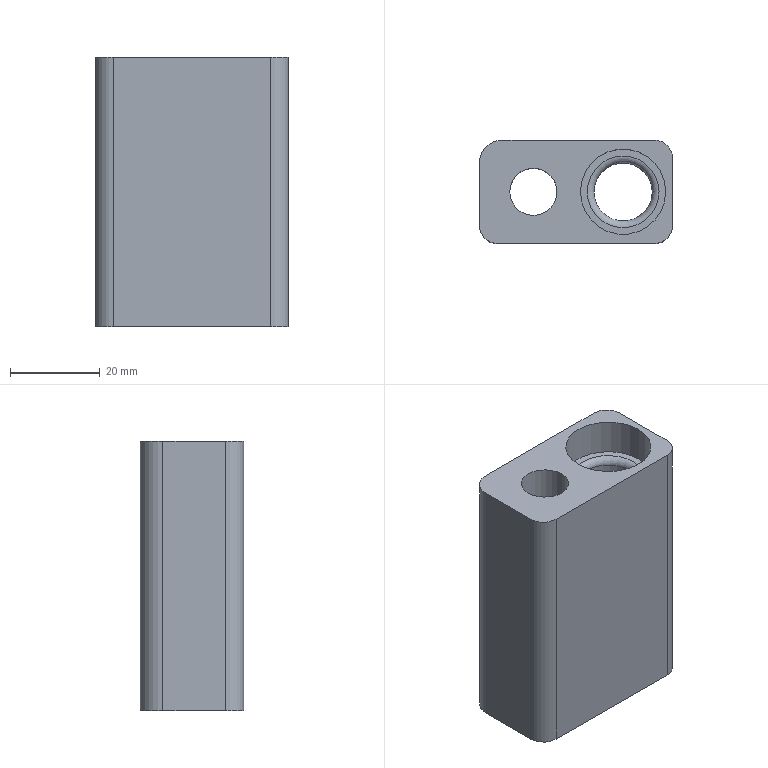Part | STEP file | gslz 2016.10.28-10_id2342_x_t | 1 solid | 17 faces | box 43 x 23 x 60 mm | volume 38390 mm3 | plane 8 | cylinder 8 | torus 1 | commonest cylinder face diameters 8 x3 10 x1 10.5 x1 13 x1 17 x1 19 x1
STEP:
#1=CARTESIAN_POINT('',(0.,0.,0.));
#2=DIRECTION('',(0.,0.,1.));
#3=DIRECTION('',(1.,0.,0.));
#4=AXIS2_PLACEMENT_3D('',#1,#2,#3);
#5=CARTESIAN_POINT('',(1124.592,-107.103,85.));
#6=VERTEX_POINT('',#5);
#7=CARTESIAN_POINT('',(1115.092,-107.103,85.));
#8=DIRECTION('',(0.,0.,1.));
#9=DIRECTION('',(1.,0.,0.));
#10=AXIS2_PLACEMENT_3D('',#7,#8,#9);
#11=CIRCLE('',#10,9.5);
#12=CARTESIAN_POINT('',(1156.092,-113.103,85.));
#13=DIRECTION('',(0.,0.,1.));
#14=DIRECTION('',(-1.,0.,0.));
#15=AXIS2_PLACEMENT_3D('',#12,#13,#14);
#16=PLANE('',#15);
#17=CARTESIAN_POINT('',(41.,-6.));
#18=DIRECTION('',(-1.,0.));
#19=AXIS2_PLACEMENT_2D('',#17,#18);
#20=CIRCLE('',#19,9.5);
#21=(GEOMETRIC_REPRESENTATION_CONTEXT(2)PARAMETRIC_REPRESENTATION_CONTEXT()REPRESENTATION_CONTEXT('',''));
#22=DEFINITIONAL_REPRESENTATION('',(#20),#21);
#23=PCURVE('',#16,#22);
#24=CARTESIAN_POINT('',(1115.092,-107.103,81.));
#25=DIRECTION('',(0.,0.,-1.));
#26=DIRECTION('',(-1.,0.,0.));
#27=AXIS2_PLACEMENT_3D('',#24,#25,#26);
#28=CYLINDRICAL_SURFACE('',#27,9.5);
#29=CARTESIAN_POINT('',(9.425,-4.));
#30=DIRECTION('',(-1.,0.));
#31=VECTOR('',#30,1.);
#32=LINE('',#29,#31);
#33=(GEOMETRIC_REPRESENTATION_CONTEXT(2)PARAMETRIC_REPRESENTATION_CONTEXT()REPRESENTATION_CONTEXT('',''));
#34=DEFINITIONAL_REPRESENTATION('',(#32),#33);
#35=PCURVE('',#28,#34);
#36=SURFACE_CURVE('',#11,(#23,#35),.PCURVE_S1.);
#37=EDGE_CURVE('',#6,#6,#36,.T.);
#38=ORIENTED_EDGE('',*,*,#37,.F.);
#39=EDGE_LOOP('',(#38));
#40=FACE_BOUND('',#39,.T.);
#41=CARTESIAN_POINT('',(1083.092,-100.603,85.));
#42=VERTEX_POINT('',#41);
#43=CARTESIAN_POINT('',(1083.092,-114.603,85.));
#44=VERTEX_POINT('',#43);
#45=CARTESIAN_POINT('',(1083.092,-113.103,85.));
#46=DIRECTION('',(0.,-1.,0.));
#47=VECTOR('',#46,1.);
#48=LINE('',#45,#47);
#49=CARTESIAN_POINT('',(73.,0.));
#50=DIRECTION('',(0.,1.));
#51=VECTOR('',#50,1.);
#52=LINE('',#49,#51);
#53=(GEOMETRIC_REPRESENTATION_CONTEXT(2)PARAMETRIC_REPRESENTATION_CONTEXT()REPRESENTATION_CONTEXT('',''));
#54=DEFINITIONAL_REPRESENTATION('',(#52),#53);
#55=PCURVE('',#16,#54);
#56=CARTESIAN_POINT('',(1083.092,-107.103,43.5));
#57=DIRECTION('',(-1.,0.,0.));
#58=DIRECTION('',(0.,0.,-1.));
#59=AXIS2_PLACEMENT_3D('',#56,#57,#58);
#60=PLANE('',#59);
#61=CARTESIAN_POINT('',(-41.5,6.));
#62=DIRECTION('',(0.,1.));
#63=VECTOR('',#62,1.);
#64=LINE('',#61,#63);
#65=(GEOMETRIC_REPRESENTATION_CONTEXT(2)PARAMETRIC_REPRESENTATION_CONTEXT()REPRESENTATION_CONTEXT('',''));
#66=DEFINITIONAL_REPRESENTATION('',(#64),#65);
#67=PCURVE('',#60,#66);
#68=SURFACE_CURVE('',#48,(#55,#67),.PCURVE_S1.);
#69=EDGE_CURVE('',#42,#44,#68,.T.);
#70=ORIENTED_EDGE('',*,*,#69,.T.);
#71=CARTESIAN_POINT('',(1087.092,-118.603,85.));
#72=VERTEX_POINT('',#71);
#73=CARTESIAN_POINT('',(1087.092,-114.603,85.));
#74=DIRECTION('',(0.,0.,1.));
#75=DIRECTION('',(1.,0.,0.));
#76=AXIS2_PLACEMENT_3D('',#73,#74,#75);
#77=CIRCLE('',#76,4.);
#78=CARTESIAN_POINT('',(69.,1.5));
#79=DIRECTION('',(-1.,0.));
#80=AXIS2_PLACEMENT_2D('',#78,#79);
#81=CIRCLE('',#80,4.);
#82=(GEOMETRIC_REPRESENTATION_CONTEXT(2)PARAMETRIC_REPRESENTATION_CONTEXT()REPRESENTATION_CONTEXT('',''));
#83=DEFINITIONAL_REPRESENTATION('',(#81),#82);
#84=PCURVE('',#16,#83);
#85=CARTESIAN_POINT('',(1087.092,-114.603,43.5));
#86=DIRECTION('',(0.,0.,-1.));
#87=DIRECTION('',(1.,0.,0.));
#88=AXIS2_PLACEMENT_3D('',#85,#86,#87);
#89=CYLINDRICAL_SURFACE('',#88,4.);
#90=CARTESIAN_POINT('',(6.283,-41.5));
#91=DIRECTION('',(-1.,0.));
#92=VECTOR('',#91,1.);
#93=LINE('',#90,#92);
#94=(GEOMETRIC_REPRESENTATION_CONTEXT(2)PARAMETRIC_REPRESENTATION_CONTEXT()REPRESENTATION_CONTEXT('',''));
#95=DEFINITIONAL_REPRESENTATION('',(#93),#94);
#96=PCURVE('',#89,#95);
#97=SURFACE_CURVE('',#77,(#84,#96),.PCURVE_S1.);
#98=EDGE_CURVE('',#44,#72,#97,.T.);
#99=ORIENTED_EDGE('',*,*,#98,.T.);
#100=CARTESIAN_POINT('',(1122.092,-118.603,85.));
#101=VERTEX_POINT('',#100);
#102=CARTESIAN_POINT('',(1198.727,-118.603,85.));
#103=DIRECTION('',(1.,0.,0.));
#104=VECTOR('',#103,1.);
#105=LINE('',#102,#104);
#106=CARTESIAN_POINT('',(-42.635,5.5));
#107=DIRECTION('',(-1.,0.));
#108=VECTOR('',#107,1.);
#109=LINE('',#106,#108);
#110=(GEOMETRIC_REPRESENTATION_CONTEXT(2)PARAMETRIC_REPRESENTATION_CONTEXT()REPRESENTATION_CONTEXT('',''));
#111=DEFINITIONAL_REPRESENTATION('',(#109),#110);
#112=PCURVE('',#16,#111);
#113=CARTESIAN_POINT('',(1198.727,-118.603,80.));
#114=DIRECTION('',(0.,1.,0.));
#115=DIRECTION('',(0.,0.,-1.));
#116=AXIS2_PLACEMENT_3D('',#113,#114,#115);
#117=PLANE('',#116);
#118=CARTESIAN_POINT('',(-5.,0.));
#119=DIRECTION('',(0.,-1.));
#120=VECTOR('',#119,1.);
#121=LINE('',#118,#120);
#122=(GEOMETRIC_REPRESENTATION_CONTEXT(2)PARAMETRIC_REPRESENTATION_CONTEXT()REPRESENTATION_CONTEXT('',''));
#123=DEFINITIONAL_REPRESENTATION('',(#121),#122);
#124=PCURVE('',#117,#123);
#125=SURFACE_CURVE('',#105,(#112,#124),.PCURVE_S1.);
#126=EDGE_CURVE('',#72,#101,#125,.T.);
#127=ORIENTED_EDGE('',*,*,#126,.T.);
#128=CARTESIAN_POINT('',(1126.092,-114.603,85.));
#129=VERTEX_POINT('',#128);
#130=CARTESIAN_POINT('',(1122.092,-114.603,85.));
#131=DIRECTION('',(0.,0.,1.));
#132=DIRECTION('',(1.,0.,0.));
#133=AXIS2_PLACEMENT_3D('',#130,#131,#132);
#134=CIRCLE('',#133,4.);
#135=CARTESIAN_POINT('',(34.,1.5));
#136=DIRECTION('',(-1.,0.));
#137=AXIS2_PLACEMENT_2D('',#135,#136);
#138=CIRCLE('',#137,4.);
#139=(GEOMETRIC_REPRESENTATION_CONTEXT(2)PARAMETRIC_REPRESENTATION_CONTEXT()REPRESENTATION_CONTEXT('',''));
#140=DEFINITIONAL_REPRESENTATION('',(#138),#139);
#141=PCURVE('',#16,#140);
#142=CARTESIAN_POINT('',(1122.092,-114.603,46.));
#143=DIRECTION('',(0.,0.,-1.));
#144=DIRECTION('',(1.,0.,0.));
#145=AXIS2_PLACEMENT_3D('',#142,#143,#144);
#146=CYLINDRICAL_SURFACE('',#145,4.);
#147=CARTESIAN_POINT('',(6.283,-39.));
#148=DIRECTION('',(-1.,0.));
#149=VECTOR('',#148,1.);
#150=LINE('',#147,#149);
#151=(GEOMETRIC_REPRESENTATION_CONTEXT(2)PARAMETRIC_REPRESENTATION_CONTEXT()REPRESENTATION_CONTEXT('',''));
#152=DEFINITIONAL_REPRESENTATION('',(#150),#151);
#153=PCURVE('',#146,#152);
#154=SURFACE_CURVE('',#134,(#141,#153),.PCURVE_S1.);
#155=EDGE_CURVE('',#101,#129,#154,.T.);
#156=ORIENTED_EDGE('',*,*,#155,.T.);
#157=CARTESIAN_POINT('',(1126.092,-99.603,85.));
#158=VERTEX_POINT('',#157);
#159=CARTESIAN_POINT('',(1126.092,-107.103,85.));
#160=DIRECTION('',(0.,1.,0.));
#161=VECTOR('',#160,1.);
#162=LINE('',#159,#161);
#163=CARTESIAN_POINT('',(30.,-6.));
#164=DIRECTION('',(0.,-1.));
#165=VECTOR('',#164,1.);
#166=LINE('',#163,#165);
#167=(GEOMETRIC_REPRESENTATION_CONTEXT(2)PARAMETRIC_REPRESENTATION_CONTEXT()REPRESENTATION_CONTEXT('',''));
#168=DEFINITIONAL_REPRESENTATION('',(#166),#167);
#169=PCURVE('',#16,#168);
#170=CARTESIAN_POINT('',(1126.092,-107.103,46.));
#171=DIRECTION('',(-1.,0.,0.));
#172=DIRECTION('',(0.,0.,-1.));
#173=AXIS2_PLACEMENT_3D('',#170,#171,#172);
#174=PLANE('',#173);
#175=CARTESIAN_POINT('',(-39.,0.));
#176=DIRECTION('',(0.,-1.));
#177=VECTOR('',#176,1.);
#178=LINE('',#175,#177);
#179=(GEOMETRIC_REPRESENTATION_CONTEXT(2)PARAMETRIC_REPRESENTATION_CONTEXT()REPRESENTATION_CONTEXT('',''));
#180=DEFINITIONAL_REPRESENTATION('',(#178),#179);
#181=PCURVE('',#174,#180);
#182=SURFACE_CURVE('',#162,(#169,#181),.PCURVE_S1.);
#183=EDGE_CURVE('',#129,#158,#182,.T.);
#184=ORIENTED_EDGE('',*,*,#183,.T.);
#185=CARTESIAN_POINT('',(1122.092,-95.603,85.));
#186=VERTEX_POINT('',#185);
#187=CARTESIAN_POINT('',(1122.092,-99.603,85.));
#188=DIRECTION('',(0.,0.,1.));
#189=DIRECTION('',(1.,0.,0.));
#190=AXIS2_PLACEMENT_3D('',#187,#188,#189);
#191=CIRCLE('',#190,4.);
#192=CARTESIAN_POINT('',(34.,-13.5));
#193=DIRECTION('',(-1.,0.));
#194=AXIS2_PLACEMENT_2D('',#192,#193);
#195=CIRCLE('',#194,4.);
#196=(GEOMETRIC_REPRESENTATION_CONTEXT(2)PARAMETRIC_REPRESENTATION_CONTEXT()REPRESENTATION_CONTEXT('',''));
#197=DEFINITIONAL_REPRESENTATION('',(#195),#196);
#198=PCURVE('',#16,#197);
#199=CARTESIAN_POINT('',(1122.092,-99.603,80.));
#200=DIRECTION('',(0.,0.,-1.));
#201=DIRECTION('',(1.,0.,0.));
#202=AXIS2_PLACEMENT_3D('',#199,#200,#201);
#203=CYLINDRICAL_SURFACE('',#202,4.);
#204=CARTESIAN_POINT('',(6.283,-5.));
#205=DIRECTION('',(-1.,0.));
#206=VECTOR('',#205,1.);
#207=LINE('',#204,#206);
#208=(GEOMETRIC_REPRESENTATION_CONTEXT(2)PARAMETRIC_REPRESENTATION_CONTEXT()REPRESENTATION_CONTEXT('',''));
#209=DEFINITIONAL_REPRESENTATION('',(#207),#208);
#210=PCURVE('',#203,#209);
#211=SURFACE_CURVE('',#191,(#198,#210),.PCURVE_S1.);
#212=EDGE_CURVE('',#158,#186,#211,.T.);
#213=ORIENTED_EDGE('',*,*,#212,.T.);
#214=CARTESIAN_POINT('',(1088.092,-95.603,85.));
#215=VERTEX_POINT('',#214);
#216=CARTESIAN_POINT('',(463.092,-95.603,85.));
#217=DIRECTION('',(-1.,0.,0.));
#218=VECTOR('',#217,1.);
#219=LINE('',#216,#218);
#220=CARTESIAN_POINT('',(693.,-17.5));
#221=DIRECTION('',(1.,0.));
#222=VECTOR('',#221,1.);
#223=LINE('',#220,#222);
#224=(GEOMETRIC_REPRESENTATION_CONTEXT(2)PARAMETRIC_REPRESENTATION_CONTEXT()REPRESENTATION_CONTEXT('',''));
#225=DEFINITIONAL_REPRESENTATION('',(#223),#224);
#226=PCURVE('',#16,#225);
#227=CARTESIAN_POINT('',(463.092,-95.603,80.));
#228=DIRECTION('',(0.,-1.,0.));
#229=DIRECTION('',(0.,0.,1.));
#230=AXIS2_PLACEMENT_3D('',#227,#228,#229);
#231=PLANE('',#230);
#232=CARTESIAN_POINT('',(5.,0.));
#233=DIRECTION('',(0.,1.));
#234=VECTOR('',#233,1.);
#235=LINE('',#232,#234);
#236=(GEOMETRIC_REPRESENTATION_CONTEXT(2)PARAMETRIC_REPRESENTATION_CONTEXT()REPRESENTATION_CONTEXT('',''));
#237=DEFINITIONAL_REPRESENTATION('',(#235),#236);
#238=PCURVE('',#231,#237);
#239=SURFACE_CURVE('',#219,(#226,#238),.PCURVE_S1.);
#240=EDGE_CURVE('',#186,#215,#239,.T.);
#241=ORIENTED_EDGE('',*,*,#240,.T.);
#242=CARTESIAN_POINT('',(1088.092,-100.603,85.));
#243=DIRECTION('',(0.,0.,1.));
#244=DIRECTION('',(1.,0.,0.));
#245=AXIS2_PLACEMENT_3D('',#242,#243,#244);
#246=CIRCLE('',#245,5.);
#247=CARTESIAN_POINT('',(68.,-12.5));
#248=DIRECTION('',(-1.,0.));
#249=AXIS2_PLACEMENT_2D('',#247,#248);
#250=CIRCLE('',#249,5.);
#251=(GEOMETRIC_REPRESENTATION_CONTEXT(2)PARAMETRIC_REPRESENTATION_CONTEXT()REPRESENTATION_CONTEXT('',''));
#252=DEFINITIONAL_REPRESENTATION('',(#250),#251);
#253=PCURVE('',#16,#252);
#254=CARTESIAN_POINT('',(1088.092,-100.603,43.5));
#255=DIRECTION('',(0.,0.,1.));
#256=DIRECTION('',(-1.,0.,0.));
#257=AXIS2_PLACEMENT_3D('',#254,#255,#256);
#258=CYLINDRICAL_SURFACE('',#257,5.);
#259=CARTESIAN_POINT('',(3.142,41.5));
#260=DIRECTION('',(1.,0.));
#261=VECTOR('',#260,1.);
#262=LINE('',#259,#261);
#263=(GEOMETRIC_REPRESENTATION_CONTEXT(2)PARAMETRIC_REPRESENTATION_CONTEXT()REPRESENTATION_CONTEXT('',''));
#264=DEFINITIONAL_REPRESENTATION('',(#262),#263);
#265=PCURVE('',#258,#264);
#266=SURFACE_CURVE('',#246,(#253,#265),.PCURVE_S1.);
#267=EDGE_CURVE('',#215,#42,#266,.T.);
#268=ORIENTED_EDGE('',*,*,#267,.T.);
#269=EDGE_LOOP('',(#70,#99,#127,#156,#184,#213,#241,#268));
#270=FACE_BOUND('',#269,.T.);
#271=CARTESIAN_POINT('',(1100.342,-107.103,85.));
#272=VERTEX_POINT('',#271);
#273=CARTESIAN_POINT('',(1095.092,-107.103,85.));
#274=DIRECTION('',(0.,0.,-1.));
#275=DIRECTION('',(1.,0.,0.));
#276=AXIS2_PLACEMENT_3D('',#273,#274,#275);
#277=CIRCLE('',#276,5.25);
#278=CARTESIAN_POINT('',(55.75,-6.));
#279=CARTESIAN_POINT('',(55.75,3.093));
#280=CARTESIAN_POINT('',(63.625,-1.453));
#281=CARTESIAN_POINT('',(71.5,-6.));
#282=CARTESIAN_POINT('',(63.625,-10.547));
#283=CARTESIAN_POINT('',(55.75,-15.093));
#284=CARTESIAN_POINT('',(55.75,-6.));
#285=(BOUNDED_CURVE()B_SPLINE_CURVE(2,(#278,#279,#280,#281,#282,#283,#284),.UNSPECIFIED.,.T.,.F.)B_SPLINE_CURVE_WITH_KNOTS((1,2,2,2,2,1),(-2.094,0.,2.094,4.189,6.283,8.378),.UNSPECIFIED.)CURVE()GEOMETRIC_REPRESENTATION_ITEM()RATIONAL_B_SPLINE_CURVE((1.,0.5,1.,0.5,1.,0.5,1.))REPRESENTATION_ITEM(''));
#286=(GEOMETRIC_REPRESENTATION_CONTEXT(2)PARAMETRIC_REPRESENTATION_CONTEXT()REPRESENTATION_CONTEXT('',''));
#287=DEFINITIONAL_REPRESENTATION('',(#285),#286);
#288=PCURVE('',#16,#287);
#289=CARTESIAN_POINT('',(1095.092,-107.103,-18.));
#290=DIRECTION('',(0.,0.,1.));
#291=DIRECTION('',(-1.,0.,0.));
#292=AXIS2_PLACEMENT_3D('',#289,#290,#291);
#293=CYLINDRICAL_SURFACE('',#292,5.25);
#294=CARTESIAN_POINT('',(9.425,103.));
#295=DIRECTION('',(-1.,0.));
#296=VECTOR('',#295,1.);
#297=LINE('',#294,#296);
#298=(GEOMETRIC_REPRESENTATION_CONTEXT(2)PARAMETRIC_REPRESENTATION_CONTEXT()REPRESENTATION_CONTEXT('',''));
#299=DEFINITIONAL_REPRESENTATION('',(#297),#298);
#300=PCURVE('',#293,#299);
#301=SURFACE_CURVE('',#277,(#288,#300),.PCURVE_S1.);
#302=EDGE_CURVE('',#272,#272,#301,.T.);
#303=ORIENTED_EDGE('',*,*,#302,.T.);
#304=EDGE_LOOP('',(#303));
#305=FACE_BOUND('',#304,.T.);
#306=ADVANCED_FACE('',(#40,#270,#305),#16,.T.);
#307=CARTESIAN_POINT('',(1108.592,-107.103,25.));
#308=VERTEX_POINT('',#307);
#309=CARTESIAN_POINT('',(1115.092,-107.103,25.));
#310=DIRECTION('',(0.,0.,1.));
#311=DIRECTION('',(-1.,0.,0.));
#312=AXIS2_PLACEMENT_3D('',#309,#310,#311);
#313=CIRCLE('',#312,6.5);
#314=CARTESIAN_POINT('',(1164.092,-53.103,25.));
#315=DIRECTION('',(0.,0.,-1.));
#316=DIRECTION('',(1.,0.,0.));
#317=AXIS2_PLACEMENT_3D('',#314,#315,#316);
#318=PLANE('',#317);
#319=CARTESIAN_POINT('',(-55.5,54.));
#320=CARTESIAN_POINT('',(-55.5,65.258));
#321=CARTESIAN_POINT('',(-45.75,59.629));
#322=CARTESIAN_POINT('',(-36.,54.));
#323=CARTESIAN_POINT('',(-45.75,48.371));
#324=CARTESIAN_POINT('',(-55.5,42.742));
#325=CARTESIAN_POINT('',(-55.5,54.));
#326=(BOUNDED_CURVE()B_SPLINE_CURVE(2,(#319,#320,#321,#322,#323,#324,#325),.UNSPECIFIED.,.T.,.F.)B_SPLINE_CURVE_WITH_KNOTS((1,2,2,2,2,1),(-2.094,0.,2.094,4.189,6.283,8.378),.UNSPECIFIED.)CURVE()GEOMETRIC_REPRESENTATION_ITEM()RATIONAL_B_SPLINE_CURVE((1.,0.5,1.,0.5,1.,0.5,1.))REPRESENTATION_ITEM(''));
#327=(GEOMETRIC_REPRESENTATION_CONTEXT(2)PARAMETRIC_REPRESENTATION_CONTEXT()REPRESENTATION_CONTEXT('',''));
#328=DEFINITIONAL_REPRESENTATION('',(#326),#327);
#329=PCURVE('',#318,#328);
#330=CARTESIAN_POINT('',(1115.092,-107.103,45.5));
#331=DIRECTION('',(0.,0.,-1.));
#332=DIRECTION('',(-1.,0.,0.));
#333=AXIS2_PLACEMENT_3D('',#330,#331,#332);
#334=CYLINDRICAL_SURFACE('',#333,6.5);
#335=CARTESIAN_POINT('',(6.283,20.5));
#336=DIRECTION('',(-1.,0.));
#337=VECTOR('',#336,1.);
#338=LINE('',#335,#337);
#339=(GEOMETRIC_REPRESENTATION_CONTEXT(2)PARAMETRIC_REPRESENTATION_CONTEXT()REPRESENTATION_CONTEXT('',''));
#340=DEFINITIONAL_REPRESENTATION('',(#338),#339);
#341=PCURVE('',#334,#340);
#342=SURFACE_CURVE('',#313,(#329,#341),.PCURVE_S1.);
#343=EDGE_CURVE('',#308,#308,#342,.T.);
#344=ORIENTED_EDGE('',*,*,#343,.T.);
#345=EDGE_LOOP('',(#344));
#346=FACE_BOUND('',#345,.T.);
#347=CARTESIAN_POINT('',(1086.592,-107.103,25.));
#348=VERTEX_POINT('',#347);
#349=CARTESIAN_POINT('',(1095.092,-107.103,25.));
#350=DIRECTION('',(0.,0.,1.));
#351=DIRECTION('',(-1.,0.,0.));
#352=AXIS2_PLACEMENT_3D('',#349,#350,#351);
#353=CIRCLE('',#352,8.5);
#354=CARTESIAN_POINT('',(-77.5,54.));
#355=CARTESIAN_POINT('',(-77.5,68.722));
#356=CARTESIAN_POINT('',(-64.75,61.361));
#357=CARTESIAN_POINT('',(-52.,54.));
#358=CARTESIAN_POINT('',(-64.75,46.639));
#359=CARTESIAN_POINT('',(-77.5,39.278));
#360=CARTESIAN_POINT('',(-77.5,54.));
#361=(BOUNDED_CURVE()B_SPLINE_CURVE(2,(#354,#355,#356,#357,#358,#359,#360),.UNSPECIFIED.,.T.,.F.)B_SPLINE_CURVE_WITH_KNOTS((1,2,2,2,2,1),(-2.094,0.,2.094,4.189,6.283,8.378),.UNSPECIFIED.)CURVE()GEOMETRIC_REPRESENTATION_ITEM()RATIONAL_B_SPLINE_CURVE((1.,0.5,1.,0.5,1.,0.5,1.))REPRESENTATION_ITEM(''));
#362=(GEOMETRIC_REPRESENTATION_CONTEXT(2)PARAMETRIC_REPRESENTATION_CONTEXT()REPRESENTATION_CONTEXT('',''));
#363=DEFINITIONAL_REPRESENTATION('',(#361),#362);
#364=PCURVE('',#318,#363);
#365=CARTESIAN_POINT('',(1095.092,-107.103,-8.));
#366=DIRECTION('',(0.,0.,1.));
#367=DIRECTION('',(-1.,0.,0.));
#368=AXIS2_PLACEMENT_3D('',#365,#366,#367);
#369=CYLINDRICAL_SURFACE('',#368,8.5);
#370=CARTESIAN_POINT('',(0.,33.));
#371=DIRECTION('',(1.,0.));
#372=VECTOR('',#371,1.);
#373=LINE('',#370,#372);
#374=(GEOMETRIC_REPRESENTATION_CONTEXT(2)PARAMETRIC_REPRESENTATION_CONTEXT()REPRESENTATION_CONTEXT('',''));
#375=DEFINITIONAL_REPRESENTATION('',(#373),#374);
#376=PCURVE('',#369,#375);
#377=SURFACE_CURVE('',#353,(#364,#376),.PCURVE_S1.);
#378=EDGE_CURVE('',#348,#348,#377,.T.);
#379=ORIENTED_EDGE('',*,*,#378,.T.);
#380=EDGE_LOOP('',(#379));
#381=FACE_BOUND('',#380,.T.);
#382=CARTESIAN_POINT('',(1087.092,-118.603,25.));
#383=VERTEX_POINT('',#382);
#384=CARTESIAN_POINT('',(1122.092,-118.603,25.));
#385=VERTEX_POINT('',#384);
#386=CARTESIAN_POINT('',(1164.092,-118.603,25.));
#387=DIRECTION('',(1.,0.,0.));
#388=VECTOR('',#387,1.);
#389=LINE('',#386,#388);
#390=CARTESIAN_POINT('',(0.,65.5));
#391=DIRECTION('',(1.,0.));
#392=VECTOR('',#391,1.);
#393=LINE('',#390,#392);
#394=(GEOMETRIC_REPRESENTATION_CONTEXT(2)PARAMETRIC_REPRESENTATION_CONTEXT()REPRESENTATION_CONTEXT('',''));
#395=DEFINITIONAL_REPRESENTATION('',(#393),#394);
#396=PCURVE('',#318,#395);
#397=CARTESIAN_POINT('',(55.,34.635));
#398=DIRECTION('',(0.,-1.));
#399=VECTOR('',#398,1.);
#400=LINE('',#397,#399);
#401=(GEOMETRIC_REPRESENTATION_CONTEXT(2)PARAMETRIC_REPRESENTATION_CONTEXT()REPRESENTATION_CONTEXT('',''));
#402=DEFINITIONAL_REPRESENTATION('',(#400),#401);
#403=PCURVE('',#117,#402);
#404=SURFACE_CURVE('',#389,(#396,#403),.PCURVE_S1.);
#405=EDGE_CURVE('',#383,#385,#404,.T.);
#406=ORIENTED_EDGE('',*,*,#405,.F.);
#407=CARTESIAN_POINT('',(1083.092,-114.603,25.));
#408=VERTEX_POINT('',#407);
#409=CARTESIAN_POINT('',(1087.092,-114.603,25.));
#410=DIRECTION('',(0.,0.,-1.));
#411=DIRECTION('',(-1.,0.,0.));
#412=AXIS2_PLACEMENT_3D('',#409,#410,#411);
#413=CIRCLE('',#412,4.);
#414=CARTESIAN_POINT('',(-77.,61.5));
#415=DIRECTION('',(-1.,0.));
#416=AXIS2_PLACEMENT_2D('',#414,#415);
#417=CIRCLE('',#416,4.);
#418=(GEOMETRIC_REPRESENTATION_CONTEXT(2)PARAMETRIC_REPRESENTATION_CONTEXT()REPRESENTATION_CONTEXT('',''));
#419=DEFINITIONAL_REPRESENTATION('',(#417),#418);
#420=PCURVE('',#318,#419);
#421=CARTESIAN_POINT('',(-3.142,18.5));
#422=DIRECTION('',(1.,0.));
#423=VECTOR('',#422,1.);
#424=LINE('',#421,#423);
#425=(GEOMETRIC_REPRESENTATION_CONTEXT(2)PARAMETRIC_REPRESENTATION_CONTEXT()REPRESENTATION_CONTEXT('',''));
#426=DEFINITIONAL_REPRESENTATION('',(#424),#425);
#427=PCURVE('',#89,#426);
#428=SURFACE_CURVE('',#413,(#420,#427),.PCURVE_S1.);
#429=EDGE_CURVE('',#383,#408,#428,.T.);
#430=ORIENTED_EDGE('',*,*,#429,.T.);
#431=CARTESIAN_POINT('',(1083.092,-100.603,25.));
#432=VERTEX_POINT('',#431);
#433=CARTESIAN_POINT('',(1083.092,-53.103,25.));
#434=DIRECTION('',(0.,1.,0.));
#435=VECTOR('',#434,1.);
#436=LINE('',#433,#435);
#437=CARTESIAN_POINT('',(-81.,0.));
#438=DIRECTION('',(0.,-1.));
#439=VECTOR('',#438,1.);
#440=LINE('',#437,#439);
#441=(GEOMETRIC_REPRESENTATION_CONTEXT(2)PARAMETRIC_REPRESENTATION_CONTEXT()REPRESENTATION_CONTEXT('',''));
#442=DEFINITIONAL_REPRESENTATION('',(#440),#441);
#443=PCURVE('',#318,#442);
#444=CARTESIAN_POINT('',(18.5,-54.));
#445=DIRECTION('',(0.,-1.));
#446=VECTOR('',#445,1.);
#447=LINE('',#444,#446);
#448=(GEOMETRIC_REPRESENTATION_CONTEXT(2)PARAMETRIC_REPRESENTATION_CONTEXT()REPRESENTATION_CONTEXT('',''));
#449=DEFINITIONAL_REPRESENTATION('',(#447),#448);
#450=PCURVE('',#60,#449);
#451=SURFACE_CURVE('',#436,(#443,#450),.PCURVE_S1.);
#452=EDGE_CURVE('',#408,#432,#451,.T.);
#453=ORIENTED_EDGE('',*,*,#452,.T.);
#454=CARTESIAN_POINT('',(1088.092,-95.603,25.));
#455=VERTEX_POINT('',#454);
#456=CARTESIAN_POINT('',(1088.092,-100.603,25.));
#457=DIRECTION('',(0.,0.,-1.));
#458=DIRECTION('',(-1.,0.,0.));
#459=AXIS2_PLACEMENT_3D('',#456,#457,#458);
#460=CIRCLE('',#459,5.);
#461=CARTESIAN_POINT('',(-76.,47.5));
#462=DIRECTION('',(-1.,0.));
#463=AXIS2_PLACEMENT_2D('',#461,#462);
#464=CIRCLE('',#463,5.);
#465=(GEOMETRIC_REPRESENTATION_CONTEXT(2)PARAMETRIC_REPRESENTATION_CONTEXT()REPRESENTATION_CONTEXT('',''));
#466=DEFINITIONAL_REPRESENTATION('',(#464),#465);
#467=PCURVE('',#318,#466);
#468=CARTESIAN_POINT('',(6.283,-18.5));
#469=DIRECTION('',(-1.,0.));
#470=VECTOR('',#469,1.);
#471=LINE('',#468,#470);
#472=(GEOMETRIC_REPRESENTATION_CONTEXT(2)PARAMETRIC_REPRESENTATION_CONTEXT()REPRESENTATION_CONTEXT('',''));
#473=DEFINITIONAL_REPRESENTATION('',(#471),#472);
#474=PCURVE('',#258,#473);
#475=SURFACE_CURVE('',#460,(#467,#474),.PCURVE_S1.);
#476=EDGE_CURVE('',#432,#455,#475,.T.);
#477=ORIENTED_EDGE('',*,*,#476,.T.);
#478=CARTESIAN_POINT('',(1122.092,-95.603,25.));
#479=VERTEX_POINT('',#478);
#480=CARTESIAN_POINT('',(1164.092,-95.603,25.));
#481=DIRECTION('',(-1.,0.,0.));
#482=VECTOR('',#481,1.);
#483=LINE('',#480,#482);
#484=CARTESIAN_POINT('',(0.,42.5));
#485=DIRECTION('',(-1.,0.));
#486=VECTOR('',#485,1.);
#487=LINE('',#484,#486);
#488=(GEOMETRIC_REPRESENTATION_CONTEXT(2)PARAMETRIC_REPRESENTATION_CONTEXT()REPRESENTATION_CONTEXT('',''));
#489=DEFINITIONAL_REPRESENTATION('',(#487),#488);
#490=PCURVE('',#318,#489);
#491=CARTESIAN_POINT('',(-55.,-701.));
#492=DIRECTION('',(0.,1.));
#493=VECTOR('',#492,1.);
#494=LINE('',#491,#493);
#495=(GEOMETRIC_REPRESENTATION_CONTEXT(2)PARAMETRIC_REPRESENTATION_CONTEXT()REPRESENTATION_CONTEXT('',''));
#496=DEFINITIONAL_REPRESENTATION('',(#494),#495);
#497=PCURVE('',#231,#496);
#498=SURFACE_CURVE('',#483,(#490,#497),.PCURVE_S1.);
#499=EDGE_CURVE('',#479,#455,#498,.T.);
#500=ORIENTED_EDGE('',*,*,#499,.F.);
#501=CARTESIAN_POINT('',(1126.092,-99.603,25.));
#502=VERTEX_POINT('',#501);
#503=CARTESIAN_POINT('',(1122.092,-99.603,25.));
#504=DIRECTION('',(0.,0.,-1.));
#505=DIRECTION('',(-1.,0.,0.));
#506=AXIS2_PLACEMENT_3D('',#503,#504,#505);
#507=CIRCLE('',#506,4.);
#508=CARTESIAN_POINT('',(-42.,46.5));
#509=DIRECTION('',(-1.,0.));
#510=AXIS2_PLACEMENT_2D('',#508,#509);
#511=CIRCLE('',#510,4.);
#512=(GEOMETRIC_REPRESENTATION_CONTEXT(2)PARAMETRIC_REPRESENTATION_CONTEXT()REPRESENTATION_CONTEXT('',''));
#513=DEFINITIONAL_REPRESENTATION('',(#511),#512);
#514=PCURVE('',#318,#513);
#515=CARTESIAN_POINT('',(3.142,55.));
#516=DIRECTION('',(1.,0.));
#517=VECTOR('',#516,1.);
#518=LINE('',#515,#517);
#519=(GEOMETRIC_REPRESENTATION_CONTEXT(2)PARAMETRIC_REPRESENTATION_CONTEXT()REPRESENTATION_CONTEXT('',''));
#520=DEFINITIONAL_REPRESENTATION('',(#518),#519);
#521=PCURVE('',#203,#520);
#522=SURFACE_CURVE('',#507,(#514,#521),.PCURVE_S1.);
#523=EDGE_CURVE('',#479,#502,#522,.T.);
#524=ORIENTED_EDGE('',*,*,#523,.T.);
#525=CARTESIAN_POINT('',(1126.092,-114.603,25.));
#526=VERTEX_POINT('',#525);
#527=CARTESIAN_POINT('',(1126.092,-107.103,25.));
#528=DIRECTION('',(0.,-1.,0.));
#529=VECTOR('',#528,1.);
#530=LINE('',#527,#529);
#531=CARTESIAN_POINT('',(-38.,54.));
#532=DIRECTION('',(0.,1.));
#533=VECTOR('',#532,1.);
#534=LINE('',#531,#533);
#535=(GEOMETRIC_REPRESENTATION_CONTEXT(2)PARAMETRIC_REPRESENTATION_CONTEXT()REPRESENTATION_CONTEXT('',''));
#536=DEFINITIONAL_REPRESENTATION('',(#534),#535);
#537=PCURVE('',#318,#536);
#538=CARTESIAN_POINT('',(21.,0.));
#539=DIRECTION('',(0.,1.));
#540=VECTOR('',#539,1.);
#541=LINE('',#538,#540);
#542=(GEOMETRIC_REPRESENTATION_CONTEXT(2)PARAMETRIC_REPRESENTATION_CONTEXT()REPRESENTATION_CONTEXT('',''));
#543=DEFINITIONAL_REPRESENTATION('',(#541),#542);
#544=PCURVE('',#174,#543);
#545=SURFACE_CURVE('',#530,(#537,#544),.PCURVE_S1.);
#546=EDGE_CURVE('',#502,#526,#545,.T.);
#547=ORIENTED_EDGE('',*,*,#546,.T.);
#548=CARTESIAN_POINT('',(1122.092,-114.603,25.));
#549=DIRECTION('',(0.,0.,-1.));
#550=DIRECTION('',(-1.,0.,0.));
#551=AXIS2_PLACEMENT_3D('',#548,#549,#550);
#552=CIRCLE('',#551,4.);
#553=CARTESIAN_POINT('',(-42.,61.5));
#554=DIRECTION('',(-1.,0.));
#555=AXIS2_PLACEMENT_2D('',#553,#554);
#556=CIRCLE('',#555,4.);
#557=(GEOMETRIC_REPRESENTATION_CONTEXT(2)PARAMETRIC_REPRESENTATION_CONTEXT()REPRESENTATION_CONTEXT('',''));
#558=DEFINITIONAL_REPRESENTATION('',(#556),#557);
#559=PCURVE('',#318,#558);
#560=CARTESIAN_POINT('',(-3.142,21.));
#561=DIRECTION('',(1.,0.));
#562=VECTOR('',#561,1.);
#563=LINE('',#560,#562);
#564=(GEOMETRIC_REPRESENTATION_CONTEXT(2)PARAMETRIC_REPRESENTATION_CONTEXT()REPRESENTATION_CONTEXT('',''));
#565=DEFINITIONAL_REPRESENTATION('',(#563),#564);
#566=PCURVE('',#146,#565);
#567=SURFACE_CURVE('',#552,(#559,#566),.PCURVE_S1.);
#568=EDGE_CURVE('',#526,#385,#567,.T.);
#569=ORIENTED_EDGE('',*,*,#568,.T.);
#570=EDGE_LOOP('',(#406,#430,#453,#477,#500,#524,#547,#569));
#571=FACE_BOUND('',#570,.T.);
#572=ADVANCED_FACE('',(#346,#381,#571),#318,.T.);
#573=ORIENTED_EDGE('',*,*,#499,.T.);
#574=CARTESIAN_POINT('',(1088.092,-95.603,95.));
#575=DIRECTION('',(0.,0.,1.));
#576=VECTOR('',#575,1.);
#577=LINE('',#574,#576);
#578=CARTESIAN_POINT('',(15.,-625.));
#579=DIRECTION('',(1.,0.));
#580=VECTOR('',#579,1.);
#581=LINE('',#578,#580);
#582=(GEOMETRIC_REPRESENTATION_CONTEXT(2)PARAMETRIC_REPRESENTATION_CONTEXT()REPRESENTATION_CONTEXT('',''));
#583=DEFINITIONAL_REPRESENTATION('',(#581),#582);
#584=PCURVE('',#231,#583);
#585=CARTESIAN_POINT('',(4.712,51.5));
#586=DIRECTION('',(0.,1.));
#587=VECTOR('',#586,1.);
#588=LINE('',#585,#587);
#589=(GEOMETRIC_REPRESENTATION_CONTEXT(2)PARAMETRIC_REPRESENTATION_CONTEXT()REPRESENTATION_CONTEXT('',''));
#590=DEFINITIONAL_REPRESENTATION('',(#588),#589);
#591=PCURVE('',#258,#590);
#592=SURFACE_CURVE('',#577,(#584,#591),.PCURVE_S1.);
#593=EDGE_CURVE('',#455,#215,#592,.T.);
#594=ORIENTED_EDGE('',*,*,#593,.T.);
#595=ORIENTED_EDGE('',*,*,#240,.F.);
#596=CARTESIAN_POINT('',(1122.092,-95.603,80.));
#597=DIRECTION('',(0.,0.,-1.));
#598=VECTOR('',#597,1.);
#599=LINE('',#596,#598);
#600=CARTESIAN_POINT('',(0.,-659.));
#601=DIRECTION('',(-1.,0.));
#602=VECTOR('',#601,1.);
#603=LINE('',#600,#602);
#604=(GEOMETRIC_REPRESENTATION_CONTEXT(2)PARAMETRIC_REPRESENTATION_CONTEXT()REPRESENTATION_CONTEXT('',''));
#605=DEFINITIONAL_REPRESENTATION('',(#603),#604);
#606=PCURVE('',#231,#605);
#607=CARTESIAN_POINT('',(4.712,0.));
#608=DIRECTION('',(0.,1.));
#609=VECTOR('',#608,1.);
#610=LINE('',#607,#609);
#611=(GEOMETRIC_REPRESENTATION_CONTEXT(2)PARAMETRIC_REPRESENTATION_CONTEXT()REPRESENTATION_CONTEXT('',''));
#612=DEFINITIONAL_REPRESENTATION('',(#610),#611);
#613=PCURVE('',#203,#612);
#614=SURFACE_CURVE('',#599,(#606,#613),.PCURVE_S1.);
#615=EDGE_CURVE('',#186,#479,#614,.T.);
#616=ORIENTED_EDGE('',*,*,#615,.T.);
#617=EDGE_LOOP('',(#573,#594,#595,#616));
#618=FACE_BOUND('',#617,.T.);
#619=ADVANCED_FACE('',(#618),#231,.F.);
#620=ORIENTED_EDGE('',*,*,#126,.F.);
#621=CARTESIAN_POINT('',(1087.092,-118.603,43.5));
#622=DIRECTION('',(0.,0.,-1.));
#623=VECTOR('',#622,1.);
#624=LINE('',#621,#623);
#625=CARTESIAN_POINT('',(36.5,111.635));
#626=DIRECTION('',(1.,0.));
#627=VECTOR('',#626,1.);
#628=LINE('',#625,#627);
#629=(GEOMETRIC_REPRESENTATION_CONTEXT(2)PARAMETRIC_REPRESENTATION_CONTEXT()REPRESENTATION_CONTEXT('',''));
#630=DEFINITIONAL_REPRESENTATION('',(#628),#629);
#631=PCURVE('',#117,#630);
#632=CARTESIAN_POINT('',(1.571,0.));
#633=DIRECTION('',(0.,1.));
#634=VECTOR('',#633,1.);
#635=LINE('',#632,#634);
#636=(GEOMETRIC_REPRESENTATION_CONTEXT(2)PARAMETRIC_REPRESENTATION_CONTEXT()REPRESENTATION_CONTEXT('',''));
#637=DEFINITIONAL_REPRESENTATION('',(#635),#636);
#638=PCURVE('',#89,#637);
#639=SURFACE_CURVE('',#624,(#631,#638),.PCURVE_S1.);
#640=EDGE_CURVE('',#72,#383,#639,.T.);
#641=ORIENTED_EDGE('',*,*,#640,.T.);
#642=ORIENTED_EDGE('',*,*,#405,.T.);
#643=CARTESIAN_POINT('',(1122.092,-118.603,80.));
#644=DIRECTION('',(0.,0.,1.));
#645=VECTOR('',#644,1.);
#646=LINE('',#643,#645);
#647=CARTESIAN_POINT('',(0.,76.635));
#648=DIRECTION('',(-1.,0.));
#649=VECTOR('',#648,1.);
#650=LINE('',#647,#649);
#651=(GEOMETRIC_REPRESENTATION_CONTEXT(2)PARAMETRIC_REPRESENTATION_CONTEXT()REPRESENTATION_CONTEXT('',''));
#652=DEFINITIONAL_REPRESENTATION('',(#650),#651);
#653=PCURVE('',#117,#652);
#654=CARTESIAN_POINT('',(1.571,-34.));
#655=DIRECTION('',(0.,-1.));
#656=VECTOR('',#655,1.);
#657=LINE('',#654,#656);
#658=(GEOMETRIC_REPRESENTATION_CONTEXT(2)PARAMETRIC_REPRESENTATION_CONTEXT()REPRESENTATION_CONTEXT('',''));
#659=DEFINITIONAL_REPRESENTATION('',(#657),#658);
#660=PCURVE('',#146,#659);
#661=SURFACE_CURVE('',#646,(#653,#660),.PCURVE_S1.);
#662=EDGE_CURVE('',#385,#101,#661,.T.);
#663=ORIENTED_EDGE('',*,*,#662,.T.);
#664=EDGE_LOOP('',(#620,#641,#642,#663));
#665=FACE_BOUND('',#664,.T.);
#666=ADVANCED_FACE('',(#665),#117,.F.);
#667=ORIENTED_EDGE('',*,*,#183,.F.);
#668=CARTESIAN_POINT('',(1126.092,-114.603,46.));
#669=DIRECTION('',(0.,0.,-1.));
#670=VECTOR('',#669,1.);
#671=LINE('',#668,#670);
#672=CARTESIAN_POINT('',(0.,7.5));
#673=DIRECTION('',(1.,0.));
#674=VECTOR('',#673,1.);
#675=LINE('',#672,#674);
#676=(GEOMETRIC_REPRESENTATION_CONTEXT(2)PARAMETRIC_REPRESENTATION_CONTEXT()REPRESENTATION_CONTEXT('',''));
#677=DEFINITIONAL_REPRESENTATION('',(#675),#676);
#678=PCURVE('',#174,#677);
#679=CARTESIAN_POINT('',(0.,0.));
#680=DIRECTION('',(0.,1.));
#681=VECTOR('',#680,1.);
#682=LINE('',#679,#681);
#683=(GEOMETRIC_REPRESENTATION_CONTEXT(2)PARAMETRIC_REPRESENTATION_CONTEXT()REPRESENTATION_CONTEXT('',''));
#684=DEFINITIONAL_REPRESENTATION('',(#682),#683);
#685=PCURVE('',#146,#684);
#686=SURFACE_CURVE('',#671,(#678,#685),.PCURVE_S1.);
#687=EDGE_CURVE('',#129,#526,#686,.T.);
#688=ORIENTED_EDGE('',*,*,#687,.T.);
#689=ORIENTED_EDGE('',*,*,#546,.F.);
#690=CARTESIAN_POINT('',(1126.092,-99.603,46.));
#691=DIRECTION('',(0.,0.,1.));
#692=VECTOR('',#691,1.);
#693=LINE('',#690,#692);
#694=CARTESIAN_POINT('',(0.,-7.5));
#695=DIRECTION('',(-1.,0.));
#696=VECTOR('',#695,1.);
#697=LINE('',#694,#696);
#698=(GEOMETRIC_REPRESENTATION_CONTEXT(2)PARAMETRIC_REPRESENTATION_CONTEXT()REPRESENTATION_CONTEXT('',''));
#699=DEFINITIONAL_REPRESENTATION('',(#697),#698);
#700=PCURVE('',#174,#699);
#701=CARTESIAN_POINT('',(6.283,34.));
#702=DIRECTION('',(0.,-1.));
#703=VECTOR('',#702,1.);
#704=LINE('',#701,#703);
#705=(GEOMETRIC_REPRESENTATION_CONTEXT(2)PARAMETRIC_REPRESENTATION_CONTEXT()REPRESENTATION_CONTEXT('',''));
#706=DEFINITIONAL_REPRESENTATION('',(#704),#705);
#707=PCURVE('',#203,#706);
#708=SURFACE_CURVE('',#693,(#700,#707),.PCURVE_S1.);
#709=EDGE_CURVE('',#502,#158,#708,.T.);
#710=ORIENTED_EDGE('',*,*,#709,.T.);
#711=EDGE_LOOP('',(#667,#688,#689,#710));
#712=FACE_BOUND('',#711,.T.);
#713=ADVANCED_FACE('',(#712),#174,.F.);
#714=ORIENTED_EDGE('',*,*,#568,.F.);
#715=ORIENTED_EDGE('',*,*,#687,.F.);
#716=ORIENTED_EDGE('',*,*,#155,.F.);
#717=ORIENTED_EDGE('',*,*,#662,.F.);
#718=EDGE_LOOP('',(#714,#715,#716,#717));
#719=FACE_BOUND('',#718,.T.);
#720=ADVANCED_FACE('',(#719),#146,.T.);
#721=ORIENTED_EDGE('',*,*,#523,.F.);
#722=ORIENTED_EDGE('',*,*,#615,.F.);
#723=ORIENTED_EDGE('',*,*,#212,.F.);
#724=ORIENTED_EDGE('',*,*,#709,.F.);
#725=EDGE_LOOP('',(#721,#722,#723,#724));
#726=FACE_BOUND('',#725,.T.);
#727=ADVANCED_FACE('',(#726),#203,.T.);
#728=CARTESIAN_POINT('',(1100.342,-107.103,65.));
#729=VERTEX_POINT('',#728);
#730=CARTESIAN_POINT('',(1095.092,-107.103,65.));
#731=DIRECTION('',(0.,0.,1.));
#732=DIRECTION('',(1.,0.,0.));
#733=AXIS2_PLACEMENT_3D('',#730,#731,#732);
#734=CIRCLE('',#733,5.25);
#735=CARTESIAN_POINT('',(3.142,83.));
#736=DIRECTION('',(1.,0.));
#737=VECTOR('',#736,1.);
#738=LINE('',#735,#737);
#739=(GEOMETRIC_REPRESENTATION_CONTEXT(2)PARAMETRIC_REPRESENTATION_CONTEXT()REPRESENTATION_CONTEXT('',''));
#740=DEFINITIONAL_REPRESENTATION('',(#738),#739);
#741=PCURVE('',#293,#740);
#742=CARTESIAN_POINT('',(422.161,-189.5,65.));
#743=DIRECTION('',(0.,0.,1.));
#744=DIRECTION('',(-1.,0.,0.));
#745=AXIS2_PLACEMENT_3D('',#742,#743,#744);
#746=PLANE('',#745);
#747=CARTESIAN_POINT('',(-672.93,-82.398));
#748=DIRECTION('',(-1.,0.));
#749=AXIS2_PLACEMENT_2D('',#747,#748);
#750=CIRCLE('',#749,5.25);
#751=(GEOMETRIC_REPRESENTATION_CONTEXT(2)PARAMETRIC_REPRESENTATION_CONTEXT()REPRESENTATION_CONTEXT('',''));
#752=DEFINITIONAL_REPRESENTATION('',(#750),#751);
#753=PCURVE('',#746,#752);
#754=SURFACE_CURVE('',#734,(#741,#753),.PCURVE_S1.);
#755=EDGE_CURVE('',#729,#729,#754,.T.);
#756=ORIENTED_EDGE('',*,*,#755,.T.);
#757=CARTESIAN_POINT('',(1100.342,-107.103,65.));
#758=CARTESIAN_POINT('',(1100.342,-107.103,85.));
#759=B_SPLINE_CURVE_WITH_KNOTS('',1,(#757,#758),.UNSPECIFIED.,.F.,.F.,(2,2),(83.,103.),.PIECEWISE_BEZIER_KNOTS.);
#760=CARTESIAN_POINT('',(9.425,0.));
#761=DIRECTION('',(0.,1.));
#762=VECTOR('',#761,1.);
#763=LINE('',#760,#762);
#764=(GEOMETRIC_REPRESENTATION_CONTEXT(2)PARAMETRIC_REPRESENTATION_CONTEXT()REPRESENTATION_CONTEXT('',''));
#765=DEFINITIONAL_REPRESENTATION('',(#763),#764);
#766=PCURVE('',#293,#765);
#767=CARTESIAN_POINT('',(3.142,0.));
#768=DIRECTION('',(0.,1.));
#769=VECTOR('',#768,1.);
#770=LINE('',#767,#769);
#771=(GEOMETRIC_REPRESENTATION_CONTEXT(2)PARAMETRIC_REPRESENTATION_CONTEXT()REPRESENTATION_CONTEXT('',''));
#772=DEFINITIONAL_REPRESENTATION('',(#770),#771);
#773=PCURVE('',#293,#772);
#774=SEAM_CURVE('',#759,(#766,#773),.PCURVE_S1.);
#775=EDGE_CURVE('',#729,#272,#774,.T.);
#776=ORIENTED_EDGE('',*,*,#775,.T.);
#777=ORIENTED_EDGE('',*,*,#302,.T.);
#778=ORIENTED_EDGE('',*,*,#775,.F.);
#779=EDGE_LOOP('',(#756,#776,#777,#778));
#780=FACE_BOUND('',#779,.F.);
#781=ADVANCED_FACE('',(#780),#293,.F.);
#782=ORIENTED_EDGE('',*,*,#755,.T.);
#783=EDGE_LOOP('',(#782));
#784=FACE_BOUND('',#783,.T.);
#785=CARTESIAN_POINT('',(1103.592,-107.103,65.));
#786=VERTEX_POINT('',#785);
#787=CARTESIAN_POINT('',(1086.592,-107.103,65.));
#788=VERTEX_POINT('',#787);
#789=CARTESIAN_POINT('',(1095.092,-107.103,65.));
#790=DIRECTION('',(0.,0.,1.));
#791=DIRECTION('',(1.,0.,0.));
#792=AXIS2_PLACEMENT_3D('',#789,#790,#791);
#793=CIRCLE('',#792,8.5);
#794=CARTESIAN_POINT('',(-672.93,-82.398));
#795=DIRECTION('',(-1.,0.));
#796=AXIS2_PLACEMENT_2D('',#794,#795);
#797=CIRCLE('',#796,8.5);
#798=(GEOMETRIC_REPRESENTATION_CONTEXT(2)PARAMETRIC_REPRESENTATION_CONTEXT()REPRESENTATION_CONTEXT('',''));
#799=DEFINITIONAL_REPRESENTATION('',(#797),#798);
#800=PCURVE('',#746,#799);
#801=CARTESIAN_POINT('',(3.142,73.));
#802=DIRECTION('',(1.,0.));
#803=VECTOR('',#802,1.);
#804=LINE('',#801,#803);
#805=(GEOMETRIC_REPRESENTATION_CONTEXT(2)PARAMETRIC_REPRESENTATION_CONTEXT()REPRESENTATION_CONTEXT('',''));
#806=DEFINITIONAL_REPRESENTATION('',(#804),#805);
#807=PCURVE('',#369,#806);
#808=SURFACE_CURVE('',#793,(#800,#807),.PCURVE_S1.);
#809=EDGE_CURVE('',#786,#788,#808,.T.);
#810=ORIENTED_EDGE('',*,*,#809,.F.);
#811=CARTESIAN_POINT('',(1095.092,-107.103,65.));
#812=DIRECTION('',(0.,0.,1.));
#813=DIRECTION('',(1.,0.,0.));
#814=AXIS2_PLACEMENT_3D('',#811,#812,#813);
#815=CIRCLE('',#814,8.5);
#816=CARTESIAN_POINT('',(-672.93,-82.398));
#817=DIRECTION('',(-1.,0.));
#818=AXIS2_PLACEMENT_2D('',#816,#817);
#819=CIRCLE('',#818,8.5);
#820=(GEOMETRIC_REPRESENTATION_CONTEXT(2)PARAMETRIC_REPRESENTATION_CONTEXT()REPRESENTATION_CONTEXT('',''));
#821=DEFINITIONAL_REPRESENTATION('',(#819),#820);
#822=PCURVE('',#746,#821);
#823=CARTESIAN_POINT('',(-3.142,73.));
#824=DIRECTION('',(1.,0.));
#825=VECTOR('',#824,1.);
#826=LINE('',#823,#825);
#827=(GEOMETRIC_REPRESENTATION_CONTEXT(2)PARAMETRIC_REPRESENTATION_CONTEXT()REPRESENTATION_CONTEXT('',''));
#828=DEFINITIONAL_REPRESENTATION('',(#826),#827);
#829=PCURVE('',#369,#828);
#830=SURFACE_CURVE('',#815,(#822,#829),.PCURVE_S1.);
#831=EDGE_CURVE('',#788,#786,#830,.T.);
#832=ORIENTED_EDGE('',*,*,#831,.F.);
#833=EDGE_LOOP('',(#810,#832));
#834=FACE_BOUND('',#833,.T.);
#835=ADVANCED_FACE('',(#784,#834),#746,.F.);
#836=ORIENTED_EDGE('',*,*,#831,.F.);
#837=CARTESIAN_POINT('',(1086.592,-107.103,25.));
#838=CARTESIAN_POINT('',(1086.592,-107.103,65.));
#839=B_SPLINE_CURVE_WITH_KNOTS('',1,(#837,#838),.UNSPECIFIED.,.F.,.F.,(2,2),(33.,73.),.PIECEWISE_BEZIER_KNOTS.);
#840=CARTESIAN_POINT('',(0.,0.));
#841=DIRECTION('',(0.,1.));
#842=VECTOR('',#841,1.);
#843=LINE('',#840,#842);
#844=(GEOMETRIC_REPRESENTATION_CONTEXT(2)PARAMETRIC_REPRESENTATION_CONTEXT()REPRESENTATION_CONTEXT('',''));
#845=DEFINITIONAL_REPRESENTATION('',(#843),#844);
#846=PCURVE('',#369,#845);
#847=CARTESIAN_POINT('',(6.283,0.));
#848=DIRECTION('',(0.,1.));
#849=VECTOR('',#848,1.);
#850=LINE('',#847,#849);
#851=(GEOMETRIC_REPRESENTATION_CONTEXT(2)PARAMETRIC_REPRESENTATION_CONTEXT()REPRESENTATION_CONTEXT('',''));
#852=DEFINITIONAL_REPRESENTATION('',(#850),#851);
#853=PCURVE('',#369,#852);
#854=SEAM_CURVE('',#839,(#846,#853),.PCURVE_S1.);
#855=EDGE_CURVE('',#348,#788,#854,.T.);
#856=ORIENTED_EDGE('',*,*,#855,.F.);
#857=ORIENTED_EDGE('',*,*,#378,.T.);
#858=ORIENTED_EDGE('',*,*,#855,.T.);
#859=ORIENTED_EDGE('',*,*,#809,.F.);
#860=EDGE_LOOP('',(#836,#856,#857,#858,#859));
#861=FACE_BOUND('',#860,.F.);
#862=ADVANCED_FACE('',(#861),#369,.F.);
#863=ORIENTED_EDGE('',*,*,#452,.F.);
#864=CARTESIAN_POINT('',(1083.092,-114.603,43.5));
#865=DIRECTION('',(0.,0.,1.));
#866=VECTOR('',#865,1.);
#867=LINE('',#864,#866);
#868=CARTESIAN_POINT('',(0.,7.5));
#869=DIRECTION('',(-1.,0.));
#870=VECTOR('',#869,1.);
#871=LINE('',#868,#870);
#872=(GEOMETRIC_REPRESENTATION_CONTEXT(2)PARAMETRIC_REPRESENTATION_CONTEXT()REPRESENTATION_CONTEXT('',''));
#873=DEFINITIONAL_REPRESENTATION('',(#871),#872);
#874=PCURVE('',#60,#873);
#875=CARTESIAN_POINT('',(3.142,0.));
#876=DIRECTION('',(0.,-1.));
#877=VECTOR('',#876,1.);
#878=LINE('',#875,#877);
#879=(GEOMETRIC_REPRESENTATION_CONTEXT(2)PARAMETRIC_REPRESENTATION_CONTEXT()REPRESENTATION_CONTEXT('',''));
#880=DEFINITIONAL_REPRESENTATION('',(#878),#879);
#881=PCURVE('',#89,#880);
#882=SURFACE_CURVE('',#867,(#874,#881),.PCURVE_S1.);
#883=EDGE_CURVE('',#408,#44,#882,.T.);
#884=ORIENTED_EDGE('',*,*,#883,.T.);
#885=ORIENTED_EDGE('',*,*,#69,.F.);
#886=CARTESIAN_POINT('',(1083.092,-100.603,45.));
#887=DIRECTION('',(0.,0.,-1.));
#888=VECTOR('',#887,1.);
#889=LINE('',#886,#888);
#890=CARTESIAN_POINT('',(-1.5,-6.5));
#891=DIRECTION('',(1.,0.));
#892=VECTOR('',#891,1.);
#893=LINE('',#890,#892);
#894=(GEOMETRIC_REPRESENTATION_CONTEXT(2)PARAMETRIC_REPRESENTATION_CONTEXT()REPRESENTATION_CONTEXT('',''));
#895=DEFINITIONAL_REPRESENTATION('',(#893),#894);
#896=PCURVE('',#60,#895);
#897=CARTESIAN_POINT('',(6.283,1.5));
#898=DIRECTION('',(0.,-1.));
#899=VECTOR('',#898,1.);
#900=LINE('',#897,#899);
#901=(GEOMETRIC_REPRESENTATION_CONTEXT(2)PARAMETRIC_REPRESENTATION_CONTEXT()REPRESENTATION_CONTEXT('',''));
#902=DEFINITIONAL_REPRESENTATION('',(#900),#901);
#903=PCURVE('',#258,#902);
#904=SURFACE_CURVE('',#889,(#896,#903),.PCURVE_S1.);
#905=EDGE_CURVE('',#42,#432,#904,.T.);
#906=ORIENTED_EDGE('',*,*,#905,.T.);
#907=EDGE_LOOP('',(#863,#884,#885,#906));
#908=FACE_BOUND('',#907,.T.);
#909=ADVANCED_FACE('',(#908),#60,.T.);
#910=CARTESIAN_POINT('',(1121.592,-107.103,75.45));
#911=VERTEX_POINT('',#910);
#912=CARTESIAN_POINT('',(1108.592,-107.103,75.45));
#913=VERTEX_POINT('',#912);
#914=CARTESIAN_POINT('',(1115.092,-107.103,75.45));
#915=DIRECTION('',(0.,0.,-1.));
#916=DIRECTION('',(1.,0.,0.));
#917=AXIS2_PLACEMENT_3D('',#914,#915,#916);
#918=CIRCLE('',#917,6.5);
#919=CARTESIAN_POINT('',(3.142,-29.95));
#920=DIRECTION('',(1.,0.));
#921=VECTOR('',#920,1.);
#922=LINE('',#919,#921);
#923=(GEOMETRIC_REPRESENTATION_CONTEXT(2)PARAMETRIC_REPRESENTATION_CONTEXT()REPRESENTATION_CONTEXT('',''));
#924=DEFINITIONAL_REPRESENTATION('',(#922),#923);
#925=PCURVE('',#334,#924);
#926=CARTESIAN_POINT('',(1115.092,-107.103,75.45));
#927=DIRECTION('',(0.,0.,1.));
#928=DIRECTION('',(-1.,0.,0.));
#929=AXIS2_PLACEMENT_3D('',#926,#927,#928);
#930=TOROIDAL_SURFACE('',#929,8.,1.5);
#931=CARTESIAN_POINT('',(9.425,9.425));
#932=DIRECTION('',(-1.,0.));
#933=VECTOR('',#932,1.);
#934=LINE('',#931,#933);
#935=(GEOMETRIC_REPRESENTATION_CONTEXT(2)PARAMETRIC_REPRESENTATION_CONTEXT()REPRESENTATION_CONTEXT('',''));
#936=DEFINITIONAL_REPRESENTATION('',(#934),#935);
#937=PCURVE('',#930,#936);
#938=SURFACE_CURVE('',#918,(#925,#937),.PCURVE_S1.);
#939=EDGE_CURVE('',#911,#913,#938,.T.);
#940=ORIENTED_EDGE('',*,*,#939,.T.);
#941=CARTESIAN_POINT('',(1108.592,-107.103,75.45));
#942=CARTESIAN_POINT('',(1108.592,-107.103,25.));
#943=B_SPLINE_CURVE_WITH_KNOTS('',1,(#941,#942),.UNSPECIFIED.,.F.,.F.,(2,2),(-29.95,20.5),.PIECEWISE_BEZIER_KNOTS.);
#944=CARTESIAN_POINT('',(6.283,0.));
#945=DIRECTION('',(0.,1.));
#946=VECTOR('',#945,1.);
#947=LINE('',#944,#946);
#948=(GEOMETRIC_REPRESENTATION_CONTEXT(2)PARAMETRIC_REPRESENTATION_CONTEXT()REPRESENTATION_CONTEXT('',''));
#949=DEFINITIONAL_REPRESENTATION('',(#947),#948);
#950=PCURVE('',#334,#949);
#951=CARTESIAN_POINT('',(0.,0.));
#952=DIRECTION('',(0.,1.));
#953=VECTOR('',#952,1.);
#954=LINE('',#951,#953);
#955=(GEOMETRIC_REPRESENTATION_CONTEXT(2)PARAMETRIC_REPRESENTATION_CONTEXT()REPRESENTATION_CONTEXT('',''));
#956=DEFINITIONAL_REPRESENTATION('',(#954),#955);
#957=PCURVE('',#334,#956);
#958=SEAM_CURVE('',#943,(#950,#957),.PCURVE_S1.);
#959=EDGE_CURVE('',#913,#308,#958,.T.);
#960=ORIENTED_EDGE('',*,*,#959,.T.);
#961=ORIENTED_EDGE('',*,*,#343,.T.);
#962=ORIENTED_EDGE('',*,*,#959,.F.);
#963=CARTESIAN_POINT('',(1115.092,-107.103,75.45));
#964=DIRECTION('',(0.,0.,-1.));
#965=DIRECTION('',(1.,0.,0.));
#966=AXIS2_PLACEMENT_3D('',#963,#964,#965);
#967=CIRCLE('',#966,6.5);
#968=CARTESIAN_POINT('',(-3.142,-29.95));
#969=DIRECTION('',(1.,0.));
#970=VECTOR('',#969,1.);
#971=LINE('',#968,#970);
#972=(GEOMETRIC_REPRESENTATION_CONTEXT(2)PARAMETRIC_REPRESENTATION_CONTEXT()REPRESENTATION_CONTEXT('',''));
#973=DEFINITIONAL_REPRESENTATION('',(#971),#972);
#974=PCURVE('',#334,#973);
#975=CARTESIAN_POINT('',(9.425,9.425));
#976=DIRECTION('',(-1.,0.));
#977=VECTOR('',#976,1.);
#978=LINE('',#975,#977);
#979=(GEOMETRIC_REPRESENTATION_CONTEXT(2)PARAMETRIC_REPRESENTATION_CONTEXT()REPRESENTATION_CONTEXT('',''));
#980=DEFINITIONAL_REPRESENTATION('',(#978),#979);
#981=PCURVE('',#930,#980);
#982=SURFACE_CURVE('',#967,(#974,#981),.PCURVE_S1.);
#983=EDGE_CURVE('',#913,#911,#982,.T.);
#984=ORIENTED_EDGE('',*,*,#983,.T.);
#985=EDGE_LOOP('',(#940,#960,#961,#962,#984));
#986=FACE_BOUND('',#985,.F.);
#987=ADVANCED_FACE('',(#986),#334,.F.);
#988=CARTESIAN_POINT('',(1124.592,-107.103,76.95));
#989=VERTEX_POINT('',#988);
#990=CARTESIAN_POINT('',(1115.092,-107.103,76.95));
#991=DIRECTION('',(0.,0.,1.));
#992=DIRECTION('',(1.,0.,0.));
#993=AXIS2_PLACEMENT_3D('',#990,#991,#992);
#994=CIRCLE('',#993,9.5);
#995=CARTESIAN_POINT('',(9.425,4.05));
#996=DIRECTION('',(-1.,0.));
#997=VECTOR('',#996,1.);
#998=LINE('',#995,#997);
#999=(GEOMETRIC_REPRESENTATION_CONTEXT(2)PARAMETRIC_REPRESENTATION_CONTEXT()REPRESENTATION_CONTEXT('',''));
#1000=DEFINITIONAL_REPRESENTATION('',(#998),#999);
#1001=PCURVE('',#28,#1000);
#1002=CARTESIAN_POINT('',(1156.092,-113.103,76.95));
#1003=DIRECTION('',(0.,0.,1.));
#1004=DIRECTION('',(-1.,0.,0.));
#1005=AXIS2_PLACEMENT_3D('',#1002,#1003,#1004);
#1006=PLANE('',#1005);
#1007=CARTESIAN_POINT('',(41.,-6.));
#1008=DIRECTION('',(-1.,0.));
#1009=AXIS2_PLACEMENT_2D('',#1007,#1008);
#1010=CIRCLE('',#1009,9.5);
#1011=(GEOMETRIC_REPRESENTATION_CONTEXT(2)PARAMETRIC_REPRESENTATION_CONTEXT()REPRESENTATION_CONTEXT('',''));
#1012=DEFINITIONAL_REPRESENTATION('',(#1010),#1011);
#1013=PCURVE('',#1006,#1012);
#1014=SURFACE_CURVE('',#994,(#1001,#1013),.PCURVE_S1.);
#1015=EDGE_CURVE('',#989,#989,#1014,.T.);
#1016=ORIENTED_EDGE('',*,*,#1015,.T.);
#1017=CARTESIAN_POINT('',(1124.592,-107.103,85.));
#1018=CARTESIAN_POINT('',(1124.592,-107.103,76.95));
#1019=B_SPLINE_CURVE_WITH_KNOTS('',1,(#1017,#1018),.UNSPECIFIED.,.F.,.F.,(2,2),(-4.,4.05),.PIECEWISE_BEZIER_KNOTS.);
#1020=CARTESIAN_POINT('',(3.142,0.));
#1021=DIRECTION('',(0.,1.));
#1022=VECTOR('',#1021,1.);
#1023=LINE('',#1020,#1022);
#1024=(GEOMETRIC_REPRESENTATION_CONTEXT(2)PARAMETRIC_REPRESENTATION_CONTEXT()REPRESENTATION_CONTEXT('',''));
#1025=DEFINITIONAL_REPRESENTATION('',(#1023),#1024);
#1026=PCURVE('',#28,#1025);
#1027=CARTESIAN_POINT('',(9.425,0.));
#1028=DIRECTION('',(0.,1.));
#1029=VECTOR('',#1028,1.);
#1030=LINE('',#1027,#1029);
#1031=(GEOMETRIC_REPRESENTATION_CONTEXT(2)PARAMETRIC_REPRESENTATION_CONTEXT()REPRESENTATION_CONTEXT('',''));
#1032=DEFINITIONAL_REPRESENTATION('',(#1030),#1031);
#1033=PCURVE('',#28,#1032);
#1034=SEAM_CURVE('',#1019,(#1026,#1033),.PCURVE_S1.);
#1035=EDGE_CURVE('',#6,#989,#1034,.T.);
#1036=ORIENTED_EDGE('',*,*,#1035,.F.);
#1037=ORIENTED_EDGE('',*,*,#37,.F.);
#1038=ORIENTED_EDGE('',*,*,#1035,.T.);
#1039=EDGE_LOOP('',(#1016,#1036,#1037,#1038));
#1040=FACE_BOUND('',#1039,.F.);
#1041=ADVANCED_FACE('',(#1040),#28,.F.);
#1042=ORIENTED_EDGE('',*,*,#939,.T.);
#1043=ORIENTED_EDGE('',*,*,#983,.T.);
#1044=CARTESIAN_POINT('',(1123.092,-107.103,76.95));
#1045=VERTEX_POINT('',#1044);
#1046=CARTESIAN_POINT('',(1123.092,-107.103,76.95));
#1047=CARTESIAN_POINT('',(1122.691,-107.103,76.95));
#1048=CARTESIAN_POINT('',(1122.3,-107.103,76.822));
#1049=CARTESIAN_POINT('',(1121.964,-107.103,76.578));
#1050=CARTESIAN_POINT('',(1121.719,-107.103,76.242));
#1051=CARTESIAN_POINT('',(1121.592,-107.103,75.851));
#1052=CARTESIAN_POINT('',(1121.592,-107.103,75.45));
#1053=(BOUNDED_CURVE()B_SPLINE_CURVE(6,(#1046,#1047,#1048,#1049,#1050,#1051,#1052),.UNSPECIFIED.,.F.,.F.)B_SPLINE_CURVE_WITH_KNOTS((7,7),(1.571,3.142),.PIECEWISE_BEZIER_KNOTS.)CURVE()GEOMETRIC_REPRESENTATION_ITEM()RATIONAL_B_SPLINE_CURVE((1.031,1.01,0.9979,0.994,0.9979,1.01,1.031))REPRESENTATION_ITEM(''));
#1054=CARTESIAN_POINT('',(3.142,6.283));
#1055=DIRECTION('',(0.,1.));
#1056=VECTOR('',#1055,1.);
#1057=LINE('',#1054,#1056);
#1058=(GEOMETRIC_REPRESENTATION_CONTEXT(2)PARAMETRIC_REPRESENTATION_CONTEXT()REPRESENTATION_CONTEXT('',''));
#1059=DEFINITIONAL_REPRESENTATION('',(#1057),#1058);
#1060=PCURVE('',#930,#1059);
#1061=CARTESIAN_POINT('',(9.425,6.283));
#1062=DIRECTION('',(0.,1.));
#1063=VECTOR('',#1062,1.);
#1064=LINE('',#1061,#1063);
#1065=(GEOMETRIC_REPRESENTATION_CONTEXT(2)PARAMETRIC_REPRESENTATION_CONTEXT()REPRESENTATION_CONTEXT('',''));
#1066=DEFINITIONAL_REPRESENTATION('',(#1064),#1065);
#1067=PCURVE('',#930,#1066);
#1068=SEAM_CURVE('',#1053,(#1060,#1067),.PCURVE_S1.);
#1069=EDGE_CURVE('',#1045,#911,#1068,.T.);
#1070=ORIENTED_EDGE('',*,*,#1069,.F.);
#1071=CARTESIAN_POINT('',(1115.092,-107.103,76.95));
#1072=DIRECTION('',(0.,0.,1.));
#1073=DIRECTION('',(1.,0.,0.));
#1074=AXIS2_PLACEMENT_3D('',#1071,#1072,#1073);
#1075=CIRCLE('',#1074,8.);
#1076=CARTESIAN_POINT('',(3.142,7.854));
#1077=DIRECTION('',(1.,0.));
#1078=VECTOR('',#1077,1.);
#1079=LINE('',#1076,#1078);
#1080=(GEOMETRIC_REPRESENTATION_CONTEXT(2)PARAMETRIC_REPRESENTATION_CONTEXT()REPRESENTATION_CONTEXT('',''));
#1081=DEFINITIONAL_REPRESENTATION('',(#1079),#1080);
#1082=PCURVE('',#930,#1081);
#1083=CARTESIAN_POINT('',(41.,-6.));
#1084=DIRECTION('',(-1.,0.));
#1085=AXIS2_PLACEMENT_2D('',#1083,#1084);
#1086=CIRCLE('',#1085,8.);
#1087=(GEOMETRIC_REPRESENTATION_CONTEXT(2)PARAMETRIC_REPRESENTATION_CONTEXT()REPRESENTATION_CONTEXT('',''));
#1088=DEFINITIONAL_REPRESENTATION('',(#1086),#1087);
#1089=PCURVE('',#1006,#1088);
#1090=SURFACE_CURVE('',#1075,(#1082,#1089),.PCURVE_S1.);
#1091=EDGE_CURVE('',#1045,#1045,#1090,.T.);
#1092=ORIENTED_EDGE('',*,*,#1091,.T.);
#1093=ORIENTED_EDGE('',*,*,#1069,.T.);
#1094=EDGE_LOOP('',(#1042,#1043,#1070,#1092,#1093));
#1095=FACE_BOUND('',#1094,.T.);
#1096=ADVANCED_FACE('',(#1095),#930,.T.);
#1097=ORIENTED_EDGE('',*,*,#1015,.T.);
#1098=EDGE_LOOP('',(#1097));
#1099=FACE_BOUND('',#1098,.T.);
#1100=ORIENTED_EDGE('',*,*,#1091,.F.);
#1101=EDGE_LOOP('',(#1100));
#1102=FACE_BOUND('',#1101,.T.);
#1103=ADVANCED_FACE('',(#1099,#1102),#1006,.T.);
#1104=ORIENTED_EDGE('',*,*,#267,.F.);
#1105=ORIENTED_EDGE('',*,*,#593,.F.);
#1106=ORIENTED_EDGE('',*,*,#476,.F.);
#1107=ORIENTED_EDGE('',*,*,#905,.F.);
#1108=EDGE_LOOP('',(#1104,#1105,#1106,#1107));
#1109=FACE_BOUND('',#1108,.T.);
#1110=ADVANCED_FACE('',(#1109),#258,.T.);
#1111=ORIENTED_EDGE('',*,*,#98,.F.);
#1112=ORIENTED_EDGE('',*,*,#883,.F.);
#1113=ORIENTED_EDGE('',*,*,#429,.F.);
#1114=ORIENTED_EDGE('',*,*,#640,.F.);
#1115=EDGE_LOOP('',(#1111,#1112,#1113,#1114));
#1116=FACE_BOUND('',#1115,.T.);
#1117=ADVANCED_FACE('',(#1116),#89,.T.);
#1118=CLOSED_SHELL('',(#306,#572,#619,#666,#713,#720,#727,#781,#835,#862,#909,#987,#1041,#1096,#1103,#1110,#1117));
#1119=MANIFOLD_SOLID_BREP('',#1118);
#1120=(LENGTH_UNIT()NAMED_UNIT(*)SI_UNIT(.MILLI.,.METRE.));
#1121=UNCERTAINTY_MEASURE_WITH_UNIT(LENGTH_MEASURE(0.000002),#1120,'','');
#1122=(NAMED_UNIT(*)PLANE_ANGLE_UNIT()SI_UNIT($,.RADIAN.));
#1123=(NAMED_UNIT(*)SI_UNIT($,.STERADIAN.)SOLID_ANGLE_UNIT());
#1124=(GEOMETRIC_REPRESENTATION_CONTEXT(3)GLOBAL_UNCERTAINTY_ASSIGNED_CONTEXT((#1121))GLOBAL_UNIT_ASSIGNED_CONTEXT((#1120,#1122,#1123))REPRESENTATION_CONTEXT('',''));
#1125=ADVANCED_BREP_SHAPE_REPRESENTATION('',(#4,#1119),#1124);